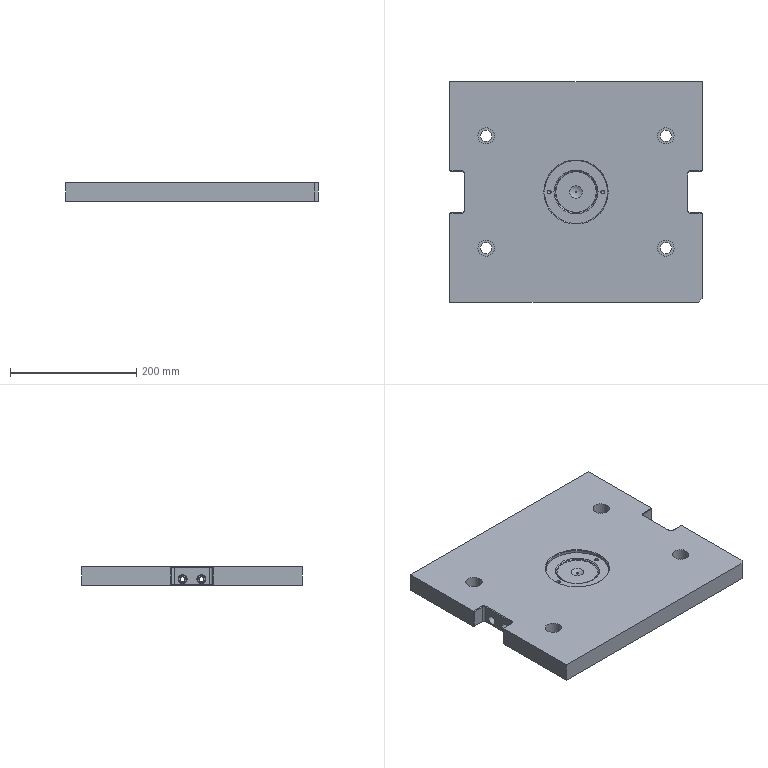Part | NX | features AD 2 | 1 solid | 125 faces | box 400 x 350 x 30 mm | volume 3966198 mm3 | plane 65 | cylinder 37 | cone 21 | sphere 1 | torus 1 | commonest cylinder face diameters 8 x11 10 x5 14 x5 20.4 x5 18 x4 26 x4